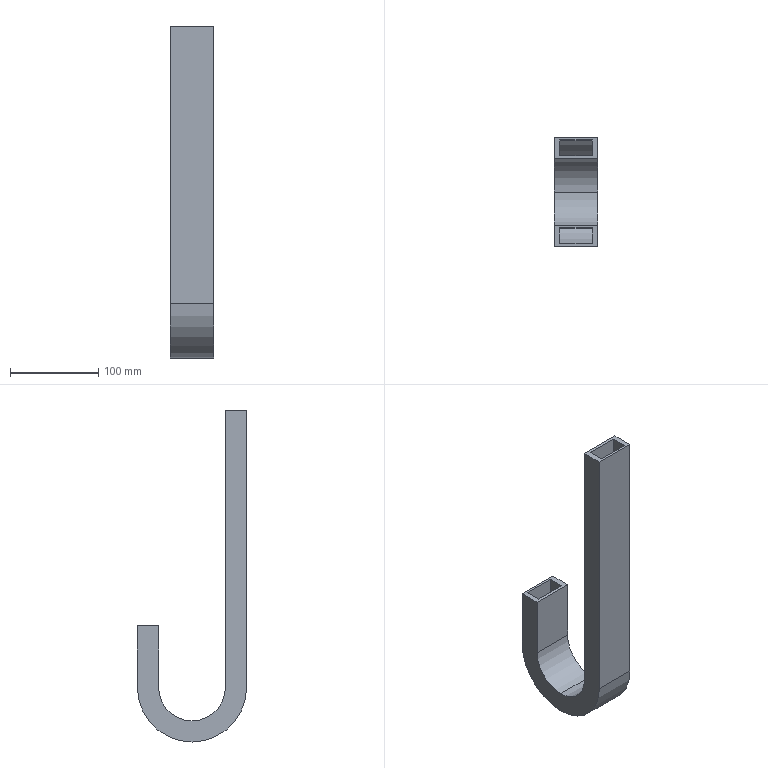Part | STEP file | 18.37.38-18-18.37.12PZ_Default | 1 solid | 22 faces | box 49 x 124 x 377 mm | volume 276461 mm3 | plane 14 | cylinder 8 | commonest cylinder face diameters 76 x2 82 x2 118 x2 124 x2